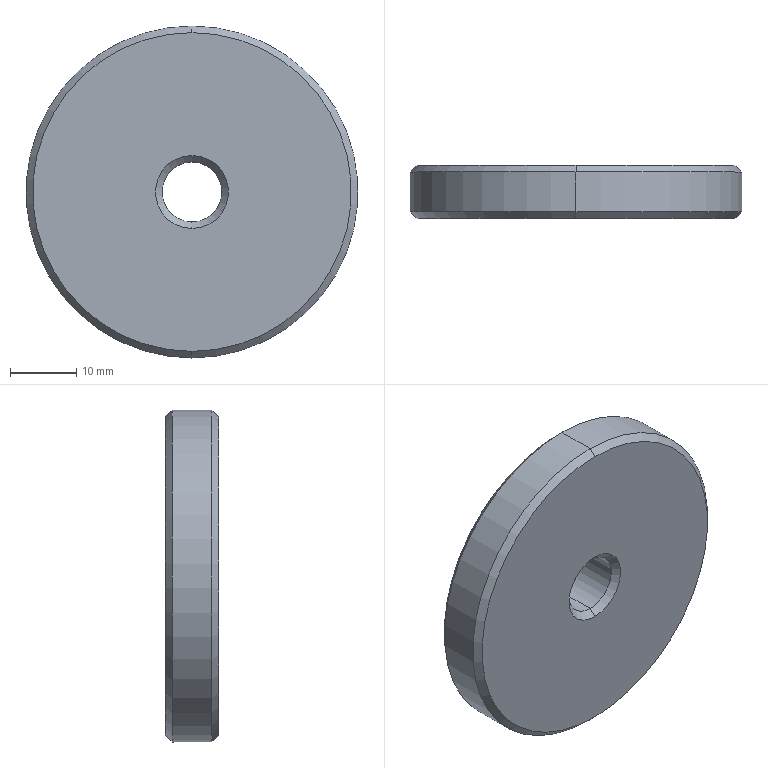Part | SolidWorks | features Revolution 1 | 1 solid | 14 faces | box 50 x 8 x 50 mm | volume 15014 mm3 | cone 8 | cylinder 4 | plane 2 | commonest cylinder face diameters 9 x2 50 x2
STEP:
#1=CARTESIAN_POINT('',(0.,7.,-25.));
#2=VERTEX_POINT('',#1);
#3=CARTESIAN_POINT('',(0.,7.,25.));
#4=VERTEX_POINT('',#3);
#5=CARTESIAN_POINT('',(0.,7.,0.));
#6=DIRECTION('',(0.,-1.,0.));
#7=DIRECTION('',(0.,0.,-1.));
#8=AXIS2_PLACEMENT_3D('',#5,#6,#7);
#9=CIRCLE('',#8,25.);
#10=EDGE_CURVE('',#2,#4,#9,.T.);
#11=ORIENTED_EDGE('',*,*,#10,.T.);
#12=CARTESIAN_POINT('',(0.,1.,25.));
#13=VERTEX_POINT('',#12);
#14=CARTESIAN_POINT('',(0.,8.,25.));
#15=DIRECTION('',(0.,-1.,0.));
#16=VECTOR('',#15,1000.);
#17=LINE('',#14,#16);
#18=EDGE_CURVE('',#4,#13,#17,.T.);
#19=ORIENTED_EDGE('',*,*,#18,.T.);
#20=CARTESIAN_POINT('',(0.,1.,-25.));
#21=VERTEX_POINT('',#20);
#22=CARTESIAN_POINT('',(0.,1.,0.));
#23=DIRECTION('',(0.,-1.,0.));
#24=DIRECTION('',(0.,0.,-1.));
#25=AXIS2_PLACEMENT_3D('',#22,#23,#24);
#26=CIRCLE('',#25,25.);
#27=EDGE_CURVE('',#21,#13,#26,.T.);
#28=ORIENTED_EDGE('',*,*,#27,.F.);
#29=CARTESIAN_POINT('',(0.,8.,-25.));
#30=DIRECTION('',(0.,-1.,0.));
#31=VECTOR('',#30,1000.);
#32=LINE('',#29,#31);
#33=EDGE_CURVE('',#2,#21,#32,.T.);
#34=ORIENTED_EDGE('',*,*,#33,.F.);
#35=EDGE_LOOP('',(#11,#19,#28,#34));
#36=FACE_OUTER_BOUND('',#35,.T.);
#37=CARTESIAN_POINT('',(0.,8.,0.));
#38=DIRECTION('',(0.,-1.,0.));
#39=DIRECTION('',(0.,0.,-1.));
#40=AXIS2_PLACEMENT_3D('',#37,#38,#39);
#41=CYLINDRICAL_SURFACE('',#40,25.);
#42=ADVANCED_FACE('',(#36),#41,.T.);
#43=CARTESIAN_POINT('',(0.,0.,-24.));
#44=VERTEX_POINT('',#43);
#45=CARTESIAN_POINT('',(0.,0.,24.));
#46=VERTEX_POINT('',#45);
#47=CARTESIAN_POINT('',(0.,0.,0.));
#48=DIRECTION('',(0.,-1.,0.));
#49=DIRECTION('',(0.,0.,-1.));
#50=AXIS2_PLACEMENT_3D('',#47,#48,#49);
#51=CIRCLE('',#50,24.);
#52=EDGE_CURVE('',#44,#46,#51,.T.);
#53=ORIENTED_EDGE('',*,*,#52,.F.);
#54=CARTESIAN_POINT('',(0.,0.,-24.));
#55=DIRECTION('',(0.,0.7071,-0.7071));
#56=VECTOR('',#55,1000.);
#57=LINE('',#54,#56);
#58=EDGE_CURVE('',#44,#21,#57,.T.);
#59=ORIENTED_EDGE('',*,*,#58,.T.);
#60=ORIENTED_EDGE('',*,*,#27,.T.);
#61=CARTESIAN_POINT('',(0.,0.,24.));
#62=DIRECTION('',(0.,0.7071,0.7071));
#63=VECTOR('',#62,1000.);
#64=LINE('',#61,#63);
#65=EDGE_CURVE('',#46,#13,#64,.T.);
#66=ORIENTED_EDGE('',*,*,#65,.F.);
#67=EDGE_LOOP('',(#53,#59,#60,#66));
#68=FACE_OUTER_BOUND('',#67,.T.);
#69=CARTESIAN_POINT('',(0.,0.,0.));
#70=DIRECTION('',(0.,1.,0.));
#71=DIRECTION('',(0.,0.,1.));
#72=AXIS2_PLACEMENT_3D('',#69,#70,#71);
#73=CONICAL_SURFACE('',#72,24.,0.7854);
#74=ADVANCED_FACE('',(#68),#73,.T.);
#75=CARTESIAN_POINT('',(0.,1.,4.5));
#76=VERTEX_POINT('',#75);
#77=CARTESIAN_POINT('',(0.,1.,-4.5));
#78=VERTEX_POINT('',#77);
#79=CARTESIAN_POINT('',(0.,1.,0.));
#80=DIRECTION('',(0.,-1.,0.));
#81=DIRECTION('',(0.,0.,-1.));
#82=AXIS2_PLACEMENT_3D('',#79,#80,#81);
#83=CIRCLE('',#82,4.5);
#84=EDGE_CURVE('',#76,#78,#83,.T.);
#85=ORIENTED_EDGE('',*,*,#84,.F.);
#86=CARTESIAN_POINT('',(0.,0.,5.5));
#87=VERTEX_POINT('',#86);
#88=CARTESIAN_POINT('',(0.,1.,4.5));
#89=DIRECTION('',(0.,-0.7071,0.7071));
#90=VECTOR('',#89,1000.);
#91=LINE('',#88,#90);
#92=EDGE_CURVE('',#76,#87,#91,.T.);
#93=ORIENTED_EDGE('',*,*,#92,.T.);
#94=CARTESIAN_POINT('',(0.,0.,-5.5));
#95=VERTEX_POINT('',#94);
#96=CARTESIAN_POINT('',(0.,0.,0.));
#97=DIRECTION('',(0.,-1.,0.));
#98=DIRECTION('',(0.,0.,-1.));
#99=AXIS2_PLACEMENT_3D('',#96,#97,#98);
#100=CIRCLE('',#99,5.5);
#101=EDGE_CURVE('',#87,#95,#100,.T.);
#102=ORIENTED_EDGE('',*,*,#101,.T.);
#103=CARTESIAN_POINT('',(0.,1.,-4.5));
#104=DIRECTION('',(0.,-0.7071,-0.7071));
#105=VECTOR('',#104,1000.);
#106=LINE('',#103,#105);
#107=EDGE_CURVE('',#78,#95,#106,.T.);
#108=ORIENTED_EDGE('',*,*,#107,.F.);
#109=EDGE_LOOP('',(#85,#93,#102,#108));
#110=FACE_OUTER_BOUND('',#109,.T.);
#111=CARTESIAN_POINT('',(0.,1.,0.));
#112=DIRECTION('',(0.,-1.,0.));
#113=DIRECTION('',(0.,0.,-1.));
#114=AXIS2_PLACEMENT_3D('',#111,#112,#113);
#115=CONICAL_SURFACE('',#114,4.5,0.7854);
#116=ADVANCED_FACE('',(#110),#115,.F.);
#117=CARTESIAN_POINT('',(0.,7.,4.5));
#118=VERTEX_POINT('',#117);
#119=CARTESIAN_POINT('',(0.,7.,-4.5));
#120=VERTEX_POINT('',#119);
#121=CARTESIAN_POINT('',(0.,7.,0.));
#122=DIRECTION('',(0.,-1.,0.));
#123=DIRECTION('',(0.,0.,-1.));
#124=AXIS2_PLACEMENT_3D('',#121,#122,#123);
#125=CIRCLE('',#124,4.5);
#126=EDGE_CURVE('',#118,#120,#125,.T.);
#127=ORIENTED_EDGE('',*,*,#126,.F.);
#128=CARTESIAN_POINT('',(0.,8.,4.5));
#129=DIRECTION('',(0.,-1.,0.));
#130=VECTOR('',#129,1000.);
#131=LINE('',#128,#130);
#132=EDGE_CURVE('',#118,#76,#131,.T.);
#133=ORIENTED_EDGE('',*,*,#132,.T.);
#134=ORIENTED_EDGE('',*,*,#84,.T.);
#135=CARTESIAN_POINT('',(0.,8.,-4.5));
#136=DIRECTION('',(0.,-1.,0.));
#137=VECTOR('',#136,1000.);
#138=LINE('',#135,#137);
#139=EDGE_CURVE('',#120,#78,#138,.T.);
#140=ORIENTED_EDGE('',*,*,#139,.F.);
#141=EDGE_LOOP('',(#127,#133,#134,#140));
#142=FACE_OUTER_BOUND('',#141,.T.);
#143=CARTESIAN_POINT('',(0.,8.,0.));
#144=DIRECTION('',(0.,-1.,0.));
#145=DIRECTION('',(0.,0.,-1.));
#146=AXIS2_PLACEMENT_3D('',#143,#144,#145);
#147=CYLINDRICAL_SURFACE('',#146,4.5);
#148=ADVANCED_FACE('',(#142),#147,.F.);
#149=ORIENTED_EDGE('',*,*,#126,.T.);
#150=CARTESIAN_POINT('',(0.,8.,-5.5));
#151=VERTEX_POINT('',#150);
#152=CARTESIAN_POINT('',(0.,8.,-5.5));
#153=DIRECTION('',(0.,0.7071,-0.7071));
#154=VECTOR('',#153,1000.);
#155=LINE('',#152,#154);
#156=EDGE_CURVE('',#120,#151,#155,.T.);
#157=ORIENTED_EDGE('',*,*,#156,.T.);
#158=CARTESIAN_POINT('',(0.,8.,5.5));
#159=VERTEX_POINT('',#158);
#160=CARTESIAN_POINT('',(0.,8.,0.));
#161=DIRECTION('',(0.,-1.,0.));
#162=DIRECTION('',(0.,0.,-1.));
#163=AXIS2_PLACEMENT_3D('',#160,#161,#162);
#164=CIRCLE('',#163,5.5);
#165=EDGE_CURVE('',#159,#151,#164,.T.);
#166=ORIENTED_EDGE('',*,*,#165,.F.);
#167=CARTESIAN_POINT('',(0.,8.,5.5));
#168=DIRECTION('',(0.,0.7071,0.7071));
#169=VECTOR('',#168,1000.);
#170=LINE('',#167,#169);
#171=EDGE_CURVE('',#118,#159,#170,.T.);
#172=ORIENTED_EDGE('',*,*,#171,.F.);
#173=EDGE_LOOP('',(#149,#157,#166,#172));
#174=FACE_OUTER_BOUND('',#173,.T.);
#175=CARTESIAN_POINT('',(0.,8.,0.));
#176=DIRECTION('',(0.,1.,0.));
#177=DIRECTION('',(0.,0.,1.));
#178=AXIS2_PLACEMENT_3D('',#175,#176,#177);
#179=CONICAL_SURFACE('',#178,5.5,0.7854);
#180=ADVANCED_FACE('',(#174),#179,.F.);
#181=CARTESIAN_POINT('',(0.,8.,-24.));
#182=VERTEX_POINT('',#181);
#183=CARTESIAN_POINT('',(0.,8.,24.));
#184=VERTEX_POINT('',#183);
#185=CARTESIAN_POINT('',(0.,8.,0.));
#186=DIRECTION('',(0.,-1.,0.));
#187=DIRECTION('',(0.,0.,-1.));
#188=AXIS2_PLACEMENT_3D('',#185,#186,#187);
#189=CIRCLE('',#188,24.);
#190=EDGE_CURVE('',#182,#184,#189,.T.);
#191=ORIENTED_EDGE('',*,*,#190,.T.);
#192=CARTESIAN_POINT('',(0.,7.,25.));
#193=DIRECTION('',(0.,-0.7071,0.7071));
#194=VECTOR('',#193,1000.);
#195=LINE('',#192,#194);
#196=EDGE_CURVE('',#184,#4,#195,.T.);
#197=ORIENTED_EDGE('',*,*,#196,.T.);
#198=ORIENTED_EDGE('',*,*,#10,.F.);
#199=CARTESIAN_POINT('',(0.,7.,-25.));
#200=DIRECTION('',(0.,-0.7071,-0.7071));
#201=VECTOR('',#200,1000.);
#202=LINE('',#199,#201);
#203=EDGE_CURVE('',#182,#2,#202,.T.);
#204=ORIENTED_EDGE('',*,*,#203,.F.);
#205=EDGE_LOOP('',(#191,#197,#198,#204));
#206=FACE_OUTER_BOUND('',#205,.T.);
#207=CARTESIAN_POINT('',(0.,7.,0.));
#208=DIRECTION('',(0.,-1.,0.));
#209=DIRECTION('',(0.,0.,-1.));
#210=AXIS2_PLACEMENT_3D('',#207,#208,#209);
#211=CONICAL_SURFACE('',#210,25.,0.7854);
#212=ADVANCED_FACE('',(#206),#211,.T.);
#213=ORIENTED_EDGE('',*,*,#196,.F.);
#214=CARTESIAN_POINT('',(0.,8.,0.));
#215=DIRECTION('',(0.,-1.,0.));
#216=DIRECTION('',(0.,0.,-1.));
#217=AXIS2_PLACEMENT_3D('',#214,#215,#216);
#218=CIRCLE('',#217,24.);
#219=EDGE_CURVE('',#184,#182,#218,.T.);
#220=ORIENTED_EDGE('',*,*,#219,.T.);
#221=ORIENTED_EDGE('',*,*,#203,.T.);
#222=CARTESIAN_POINT('',(0.,7.,0.));
#223=DIRECTION('',(0.,-1.,0.));
#224=DIRECTION('',(0.,0.,-1.));
#225=AXIS2_PLACEMENT_3D('',#222,#223,#224);
#226=CIRCLE('',#225,25.);
#227=EDGE_CURVE('',#4,#2,#226,.T.);
#228=ORIENTED_EDGE('',*,*,#227,.F.);
#229=EDGE_LOOP('',(#213,#220,#221,#228));
#230=FACE_OUTER_BOUND('',#229,.T.);
#231=CARTESIAN_POINT('',(0.,7.,0.));
#232=DIRECTION('',(0.,-1.,0.));
#233=DIRECTION('',(0.,0.,-1.));
#234=AXIS2_PLACEMENT_3D('',#231,#232,#233);
#235=CONICAL_SURFACE('',#234,25.,0.7854);
#236=ADVANCED_FACE('',(#230),#235,.T.);
#237=ORIENTED_EDGE('',*,*,#165,.T.);
#238=CARTESIAN_POINT('',(0.,8.,0.));
#239=DIRECTION('',(0.,-1.,0.));
#240=DIRECTION('',(0.,0.,-1.));
#241=AXIS2_PLACEMENT_3D('',#238,#239,#240);
#242=CIRCLE('',#241,5.5);
#243=EDGE_CURVE('',#151,#159,#242,.T.);
#244=ORIENTED_EDGE('',*,*,#243,.T.);
#245=EDGE_LOOP('',(#237,#244));
#246=FACE_BOUND('',#245,.T.);
#247=ORIENTED_EDGE('',*,*,#190,.F.);
#248=ORIENTED_EDGE('',*,*,#219,.F.);
#249=EDGE_LOOP('',(#247,#248));
#250=FACE_OUTER_BOUND('',#249,.T.);
#251=CARTESIAN_POINT('',(24.,8.,0.));
#252=DIRECTION('',(0.,1.,0.));
#253=DIRECTION('',(0.,0.,1.));
#254=AXIS2_PLACEMENT_3D('',#251,#252,#253);
#255=PLANE('',#254);
#256=ADVANCED_FACE('',(#246,#250),#255,.T.);
#257=ORIENTED_EDGE('',*,*,#156,.F.);
#258=CARTESIAN_POINT('',(0.,7.,0.));
#259=DIRECTION('',(0.,-1.,0.));
#260=DIRECTION('',(0.,0.,-1.));
#261=AXIS2_PLACEMENT_3D('',#258,#259,#260);
#262=CIRCLE('',#261,4.5);
#263=EDGE_CURVE('',#120,#118,#262,.T.);
#264=ORIENTED_EDGE('',*,*,#263,.T.);
#265=ORIENTED_EDGE('',*,*,#171,.T.);
#266=ORIENTED_EDGE('',*,*,#243,.F.);
#267=EDGE_LOOP('',(#257,#264,#265,#266));
#268=FACE_OUTER_BOUND('',#267,.T.);
#269=CARTESIAN_POINT('',(0.,8.,0.));
#270=DIRECTION('',(0.,1.,0.));
#271=DIRECTION('',(0.,0.,1.));
#272=AXIS2_PLACEMENT_3D('',#269,#270,#271);
#273=CONICAL_SURFACE('',#272,5.5,0.7854);
#274=ADVANCED_FACE('',(#268),#273,.F.);
#275=ORIENTED_EDGE('',*,*,#132,.F.);
#276=ORIENTED_EDGE('',*,*,#263,.F.);
#277=ORIENTED_EDGE('',*,*,#139,.T.);
#278=CARTESIAN_POINT('',(0.,1.,0.));
#279=DIRECTION('',(0.,-1.,0.));
#280=DIRECTION('',(0.,0.,-1.));
#281=AXIS2_PLACEMENT_3D('',#278,#279,#280);
#282=CIRCLE('',#281,4.5);
#283=EDGE_CURVE('',#78,#76,#282,.T.);
#284=ORIENTED_EDGE('',*,*,#283,.T.);
#285=EDGE_LOOP('',(#275,#276,#277,#284));
#286=FACE_OUTER_BOUND('',#285,.T.);
#287=CARTESIAN_POINT('',(0.,8.,0.));
#288=DIRECTION('',(0.,-1.,0.));
#289=DIRECTION('',(0.,0.,-1.));
#290=AXIS2_PLACEMENT_3D('',#287,#288,#289);
#291=CYLINDRICAL_SURFACE('',#290,4.5);
#292=ADVANCED_FACE('',(#286),#291,.F.);
#293=ORIENTED_EDGE('',*,*,#92,.F.);
#294=ORIENTED_EDGE('',*,*,#283,.F.);
#295=ORIENTED_EDGE('',*,*,#107,.T.);
#296=CARTESIAN_POINT('',(0.,0.,0.));
#297=DIRECTION('',(0.,-1.,0.));
#298=DIRECTION('',(0.,0.,-1.));
#299=AXIS2_PLACEMENT_3D('',#296,#297,#298);
#300=CIRCLE('',#299,5.5);
#301=EDGE_CURVE('',#95,#87,#300,.T.);
#302=ORIENTED_EDGE('',*,*,#301,.T.);
#303=EDGE_LOOP('',(#293,#294,#295,#302));
#304=FACE_OUTER_BOUND('',#303,.T.);
#305=CARTESIAN_POINT('',(0.,1.,0.));
#306=DIRECTION('',(0.,-1.,0.));
#307=DIRECTION('',(0.,0.,-1.));
#308=AXIS2_PLACEMENT_3D('',#305,#306,#307);
#309=CONICAL_SURFACE('',#308,4.5,0.7854);
#310=ADVANCED_FACE('',(#304),#309,.F.);
#311=CARTESIAN_POINT('',(0.,0.,0.));
#312=DIRECTION('',(0.,-1.,0.));
#313=DIRECTION('',(0.,0.,-1.));
#314=AXIS2_PLACEMENT_3D('',#311,#312,#313);
#315=CIRCLE('',#314,24.);
#316=EDGE_CURVE('',#46,#44,#315,.T.);
#317=ORIENTED_EDGE('',*,*,#316,.T.);
#318=ORIENTED_EDGE('',*,*,#52,.T.);
#319=EDGE_LOOP('',(#317,#318));
#320=FACE_OUTER_BOUND('',#319,.T.);
#321=ORIENTED_EDGE('',*,*,#301,.F.);
#322=ORIENTED_EDGE('',*,*,#101,.F.);
#323=EDGE_LOOP('',(#321,#322));
#324=FACE_BOUND('',#323,.T.);
#325=CARTESIAN_POINT('',(5.5,0.,0.));
#326=DIRECTION('',(0.,-1.,0.));
#327=DIRECTION('',(0.,0.,-1.));
#328=AXIS2_PLACEMENT_3D('',#325,#326,#327);
#329=PLANE('',#328);
#330=ADVANCED_FACE('',(#320,#324),#329,.T.);
#331=ORIENTED_EDGE('',*,*,#58,.F.);
#332=ORIENTED_EDGE('',*,*,#316,.F.);
#333=ORIENTED_EDGE('',*,*,#65,.T.);
#334=CARTESIAN_POINT('',(0.,1.,0.));
#335=DIRECTION('',(0.,-1.,0.));
#336=DIRECTION('',(0.,0.,-1.));
#337=AXIS2_PLACEMENT_3D('',#334,#335,#336);
#338=CIRCLE('',#337,25.);
#339=EDGE_CURVE('',#13,#21,#338,.T.);
#340=ORIENTED_EDGE('',*,*,#339,.T.);
#341=EDGE_LOOP('',(#331,#332,#333,#340));
#342=FACE_OUTER_BOUND('',#341,.T.);
#343=CARTESIAN_POINT('',(0.,0.,0.));
#344=DIRECTION('',(0.,1.,0.));
#345=DIRECTION('',(0.,0.,1.));
#346=AXIS2_PLACEMENT_3D('',#343,#344,#345);
#347=CONICAL_SURFACE('',#346,24.,0.7854);
#348=ADVANCED_FACE('',(#342),#347,.T.);
#349=ORIENTED_EDGE('',*,*,#18,.F.);
#350=ORIENTED_EDGE('',*,*,#227,.T.);
#351=ORIENTED_EDGE('',*,*,#33,.T.);
#352=ORIENTED_EDGE('',*,*,#339,.F.);
#353=EDGE_LOOP('',(#349,#350,#351,#352));
#354=FACE_OUTER_BOUND('',#353,.T.);
#355=CARTESIAN_POINT('',(0.,8.,0.));
#356=DIRECTION('',(0.,-1.,0.));
#357=DIRECTION('',(0.,0.,-1.));
#358=AXIS2_PLACEMENT_3D('',#355,#356,#357);
#359=CYLINDRICAL_SURFACE('',#358,25.);
#360=ADVANCED_FACE('',(#354),#359,.T.);
#361=CLOSED_SHELL('',(#42,#74,#116,#148,#180,#212,#236,#256,#274,#292,#310,#330,#348,#360));
#362=MANIFOLD_SOLID_BREP('',#361);
#363=CARTESIAN_POINT('',(0.,0.,0.));
#364=DIRECTION('',(0.,0.,1.));
#365=DIRECTION('',(1.,0.,0.));
#366=AXIS2_PLACEMENT_3D('',#363,#364,#365);
#367=(LENGTH_UNIT()NAMED_UNIT(*)SI_UNIT(.MILLI.,.METRE.));
#368=UNCERTAINTY_MEASURE_WITH_UNIT(LENGTH_MEASURE(0.00001),#367,'','');
#369=(NAMED_UNIT(*)PLANE_ANGLE_UNIT()SI_UNIT($,.RADIAN.));
#370=(NAMED_UNIT(*)SI_UNIT($,.STERADIAN.)SOLID_ANGLE_UNIT());
#371=(GEOMETRIC_REPRESENTATION_CONTEXT(3)GLOBAL_UNCERTAINTY_ASSIGNED_CONTEXT((#368))GLOBAL_UNIT_ASSIGNED_CONTEXT((#367,#369,#370))REPRESENTATION_CONTEXT('',''));
#372=ADVANCED_BREP_SHAPE_REPRESENTATION('',(#362,#366),#371);